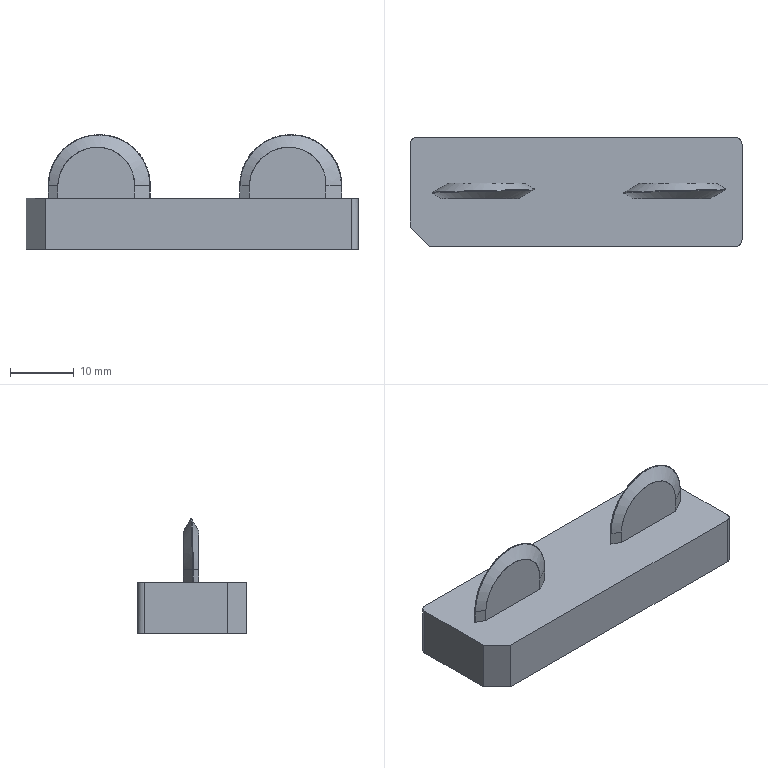NC program | PowerMill | posted with a generic post | part box 52 x 17 x 17.993 mm
Lines 9462 to 10240 of 175197:
N9559 M6
N9560 S8500 M03
N9561 G00 G90 X0.0 Y0.0
N9562 G43 Z9.7641 H3
N9563
N9564 G05 P10000 R8
N9565 X36.768 Y-7.8501
N9566 Z-8.99
N9567 G01 Z-10.19 F360.0
N9568 X31.4975 Y-7.6334 F600.0
N9569 Y0.5653
N9570 X28.8586 Y0.5675
N9571 X28.8583 Y0.2837
N9572 X28.8431 Y0.0
N9573 X28.8133 Y-0.2838
N9574 X28.7684 Y-0.5675
N9575 G02 X28.647 Y-1.0826 I-6.5218 J1.2655
N9576 G01 X28.5384 Y-1.4187
N9577 X28.4277 Y-1.7025
N9578 X28.2983 Y-1.9862
N9579 X28.1626 Y-2.2445
N9580 X28.0088 Y-2.5028
N9581 X27.779 Y-2.8375
N9582 X27.5532 Y-3.1213
N9583 X27.4447 Y-3.2451
N9584 X27.2187 Y-3.4806
N9585 X26.9945 Y-3.6887
N9586 X26.8771 Y-3.7891
N9587 X26.5942 Y-4.0081
N9588 X26.4095 Y-4.1344
N9589 X26.2217 Y-4.2562
N9590 X24.8539 Y-5.0498
N9591 X23.4821 Y-5.8366
N9592 X23.2337 Y-5.9587
N9593 X22.9163 Y-6.0931
N9594 X22.6334 Y-6.1934
N9595 X22.3504 Y-6.2763
N9596 X22.0675 Y-6.3429
N9597 X21.7846 Y-6.3935
N9598 X21.5017 Y-6.429
N9599 X21.2187 Y-6.4492
N9600 X20.6529 Y-6.455
N9601 X9.3363
N9602 X8.7704 Y-6.4517
N9603 X8.4875 Y-6.4344
N9604 X8.2046 Y-6.4021
N9605 G02 X7.6388 Y-6.2913 I0.9473 J6.3356
N9606 G01 X7.3558 Y-6.2118
N9607 X7.0602 Y-6.1105
N9608 X6.6972 Y-5.9588
N9609 X6.5071 Y-5.8667
N9610 X5.9412 Y-5.5486
N9611 X4.6897 Y-4.8238
N9612 X4.4667 Y-4.6794
N9613 X4.2437 Y-4.5184
N9614 X4.0631 Y-4.3751
N9615 X1.0968 Y-8.1713
N9616 G02 X0.7451 Y-9.1929 I-0.3518 J-0.4502
N9617 G01 X-0.7145 Y-9.193
N9618 G02 X-0.9257 Y-8.1556 I0.0 J0.5402
N9619 G01 X-0.3805 Y-7.924
N9620 G02 X0.5431 Y-7.9197 I0.467 J-1.0993
N9621 G01 X0.9635 Y-8.0936
N9622 G02 X1.0968 Y-8.1713 I-0.2185 J-0.528
N9623 G01 X4.0631 Y-4.3751
N9624 X3.923 Y-4.2563
N9625 X3.6779 Y-4.0257
N9626 X3.5166 Y-3.8572
N9627 X3.3685 Y-3.6887
N9628 G02 X2.9013 Y-3.0435 I4.0912 J3.4539
N9629 G01 X2.7769 Y-2.8375
N9630 X2.6286 Y-2.5538
N9631 X2.5463 Y-2.3764
N9632 X2.3904 Y-1.9863
N9633 G02 X2.2225 Y-1.4188 I6.0815 J2.1086
N9634 G01 X2.1632 Y-1.135
N9635 X2.1194 Y-0.8513
N9636 X2.0903 Y-0.5675
N9637 X2.076 Y-0.2838
N9638 X2.0764 Y0.0
N9639 X2.092 Y0.2838
N9640 X2.1225 Y0.5675
N9641 X2.1675 Y0.8512
N9642 X2.2278 Y1.135
N9643 X2.3048 Y1.4188
N9644 X2.3985 Y1.7025
N9645 X2.5098 Y1.9862
N9646 X2.6602 Y2.312
N9647 X2.7894 Y2.5537
N9648 G02 X3.1602 Y3.1213 I5.3365 J-3.0817
N9649 G01 X3.3863 Y3.405
N9650 X3.6779 Y3.7209
N9651 X3.9608 Y3.984
N9652 X4.2437 Y4.2144
N9653 G02 X4.8198 Y4.598 I3.727 J-4.9725
N9654 G01 X7.3959 Y6.0848
N9655 X7.6388 Y6.212
N9656 X7.9217 Y6.3406
N9657 X8.2046 Y6.4501
N9658 X8.3813 Y6.5085
N9659 X8.7704 Y6.6166
N9660 X9.0533 Y6.6754
N9661 X9.3362 Y6.7186
N9662 G02 X9.9021 Y6.7599 I0.7394 J-6.2346
N9663 G01 X21.7846 Y6.761
N9664 G02 X22.3504 Y6.7446 I0.0747 J-7.2155
N9665 G01 X22.6333 Y6.715
N9666 X22.9162 Y6.6701
N9667 G02 X23.5042 Y6.5262 I-1.2454 J-6.3649
N9668 G01 X23.776 Y6.4356
N9669 X24.0479 Y6.3281
N9670 X24.3308 Y6.1976
N9671 X24.6137 Y6.0466
N9672 X25.4638 Y5.5561
N9673 X26.3113 Y5.0612
N9674 X26.6561 Y4.8237
N9675 G02 X27.0908 Y4.4638 I-3.752 J-4.974
N9676 G01 X27.3045 Y4.2562
N9677 G02 X27.7869 Y3.6887 I-4.1486 J-4.0151
N9678 G01 X28.0087 Y3.3654
N9679 X28.1549 Y3.1213
N9680 X28.3041 Y2.8375
N9681 X28.4328 Y2.5538
N9682 X28.5746 Y2.178
N9683 X28.6354 Y1.9862
N9684 X28.7108 Y1.7025
N9685 X28.7708 Y1.4187
N9686 X28.8151 Y1.135
N9687 X28.8442 Y0.8512
N9688 X28.8586 Y0.5675
N9689 X31.4975 Y0.5653
N9690 G00 Z2.801
N9691 G01 X-36.768 Y7.8503 F10000.0
N9692 G00 Z-8.99
N9693 G01 Z-10.19 F360.0
N9694 X-31.4975 Y7.6335 F600.0
N9695 Y-0.5128
N9696 X-27.9215 Y-0.3548
N9697 X-27.9235 Y0.0
N9698 X-27.9079 Y0.2838
N9699 G02 X-27.8325 Y0.8513 I6.9347 J-0.6328
N9700 G01 X-27.7721 Y1.135
N9701 X-27.6952 Y1.4188
N9702 X-27.6015 Y1.7025
N9703 X-27.4905 Y1.9863
N9704 X-27.3336 Y2.324
N9705 G02 X-27.0541 Y2.8122 I5.6458 J-2.9085
N9706 G01 X-26.8398 Y3.1213
N9707 X-26.6139 Y3.405
N9708 X-26.3113 Y3.7317
N9709 X-26.0283 Y3.9934
N9710 X-25.7004 Y4.2563
N9711 X-25.44 Y4.438
N9712 X-25.1796 Y4.5982
N9713 X-22.5879 Y6.0946
N9714 X-22.4317 Y6.176
N9715 X-22.0675 Y6.3451
N9716 X-21.7846 Y6.4536
N9717 X-21.5636 Y6.5263
N9718 X-21.2188 Y6.6191
N9719 X-20.9358 Y6.6774
N9720 X-20.6529 Y6.7199
N9721 X-20.37 Y6.7475
N9722 X-20.1737 Y6.7568
N9723 X-19.5212 Y6.761
N9724 X-7.9217 Y6.7588
N9725 G02 X-7.3558 Y6.7135 I-0.2268 J-6.3843
N9726 G01 X-7.0729 Y6.6681
N9727 X-6.7866 Y6.6061
N9728 X-6.5071 Y6.5299
N9729 G02 X-5.9413 Y6.3234 I-1.9215 J-6.1454
N9730 G01 X-5.6583 Y6.1923
N9731 X-5.3754 Y6.0405
N9732 X-4.5252 Y5.55
N9733 X-3.6779 Y5.0543
N9734 X-3.3442 Y4.8237
N9735 X-3.0821 Y4.6152
N9736 X-2.9759 Y4.5221
N9737 X0.1585 Y8.1619
N9738 G02 X-0.0446 Y8.5772 I0.3827 J0.4444
N9739 G02 X0.5412 Y9.1928 I0.5858 J0.0291
N9740 G01 X1.205 Y9.1929
N9741 G02 X1.2599 Y8.0885 I0.0001 J-0.5536
N9742 G01 X0.5994 Y8.0227
N9743 G02 X0.1585 Y8.1619 I-0.0582 J0.5836
N9744 G01 X-2.9759 Y4.5221
N9745 X-2.9038 Y4.459
N9746 X-2.7215 Y4.2814
N9747 X-2.5463 Y4.0969
N9748 X-2.3711 Y3.8928
N9749 X-2.213 Y3.6887
N9750 X-1.9804 Y3.3482
N9751 X-1.8453 Y3.1213
N9752 X-1.6958 Y2.8375
N9753 X-1.5671 Y2.5537
N9754 X-1.4146 Y2.1456
N9755 X-1.3495 Y1.9287
N9756 X-1.2892 Y1.7025
N9757 X-1.2292 Y1.4187
N9758 X-1.1848 Y1.135
N9759 G02 X-1.1413 Y0.5675 I-6.6145 J-0.7918
N9760 G01 X-1.1416 Y0.2837
N9761 X-1.1569 Y0.0
N9762 G02 X-1.2314 Y-0.5675 I-6.5663 J0.5736
N9763 G01 X-1.2922 Y-0.8513
N9764 X-1.4146 Y-1.2813
N9765 X-1.4618 Y-1.4188
N9766 X-1.5722 Y-1.7025
N9767 X-1.7019 Y-1.9863
N9768 X-1.8325 Y-2.2359
N9769 X-2.0238 Y-2.5537
N9770 X-2.2209 Y-2.8375
N9771 X-2.4468 Y-3.1212
N9772 X-2.5463 Y-3.2349
N9773 X-2.7759 Y-3.4753
N9774 X-3.0054 Y-3.6888
N9775 X-3.1121 Y-3.7802
N9776 X-3.395 Y-4.0004
N9777 X-3.6779 Y-4.1939
N9778 X-3.878 Y-4.3143
N9779 X-5.191 Y-5.0752
N9780 X-6.5071 Y-5.8307
N9781 X-6.7665 Y-5.9588
N9782 X-7.0729 Y-6.0887
N9783 X-7.3558 Y-6.1896
N9784 X-7.6388 Y-6.2733
N9785 G02 X-8.2046 Y-6.3919 I-1.5816 J6.1369
N9786 G01 X-8.4875 Y-6.428
N9787 X-8.7704 Y-6.4489
N9788 X-9.3362 Y-6.455
N9789 X-20.6529
N9790 X-21.2188 Y-6.452
N9791 X-21.5017 Y-6.4354
N9792 G02 X-22.0675 Y-6.3568 I0.6091 J6.4567
N9793 G01 X-22.3504 Y-6.294
N9794 X-22.6334 Y-6.215
N9795 X-22.9163 Y-6.1192
N9796 X-23.3028 Y-5.9587
N9797 X-23.4821 Y-5.872
N9798 X-24.0479 Y-5.5547
N9799 X-25.3103 Y-4.8237
N9800 G02 X-26.1003 Y-4.2343 I2.9388 J4.7633
N9801 G01 X-26.3113 Y-4.0365
N9802 X-26.4747 Y-3.8656
N9803 X-26.6318 Y-3.6887
N9804 X-26.8771 Y-3.3756
N9805 X-27.0517 Y-3.1212
N9806 X-27.2229 Y-2.8375
N9807 X-27.3714 Y-2.5538
N9808 X-27.4429 Y-2.4005
N9809 X-27.5313 Y-2.1934
N9810 X-27.6095 Y-1.9863
N9811 X-27.7146 Y-1.6547
N9812 X-27.7775 Y-1.4187
N9813 X-27.8367 Y-1.135
N9814 X-27.8806 Y-0.8512
N9815 X-27.9057 Y-0.6034
N9816 X-27.9215 Y-0.3548
N9817 X-31.4975 Y-0.5128
N9818 G00 Z9.7641
N9819 G05 P0
N9820 (---------------)
N9821 ( END TOOLPATH : 精公基准台01-基准面偏置-D10 )
N9822 (---------------)
N9823 ( START TOOLPATH : 精公基准台01-基准台侧光-D10 )
N9824 (---------------)
N9825 G00 X0.0 Y0.0 Z9.7641
N9826 G05 P10000 R8
N9827 X30.2044 Y-17.2786
N9828 Z-16.89
N9829 G01 Z-18.09 F360.0
N9830 G03 X27.8526 Y-12.8662 I-1.1759 J2.2062 F600.0
N9831 G01 X27.7004 Y-12.9474
N9832 X27.6983 Y-12.9485
N9833 X27.6961 Y-12.9495
N9834 X27.38 Y-13.0947
N9835 X27.3779 Y-13.0957
N9836 X27.3758 Y-13.0965
N9837 X27.0597 Y-13.2205
N9838 X27.0576 Y-13.2213
N9839 X27.0554 Y-13.222
N9840 X26.7393 Y-13.3259
N9841 X26.7379 Y-13.3263
N9842 X26.7365 Y-13.3268
N9843 X26.6385 Y-13.355
N9844 X26.6375 Y-13.3553
N9845 X26.6364 Y-13.3555
N9846 X26.4183 Y-13.4122
N9847 X26.4164 Y-13.4127
N9848 X26.4146 Y-13.4131
N9849 X26.0984 Y-13.4794
N9850 X26.0965 Y-13.4798
N9851 X26.0945 Y-13.4802
N9852 X25.7783 Y-13.53
N9853 X25.7761 Y-13.5303
N9854 X25.7739 Y-13.5305
N9855 X25.4577 Y-13.5623
N9856 X25.4557 Y-13.5624
N9857 X25.4537 Y-13.5626
N9858 X25.1375 Y-13.5781
N9859 X25.1358 Y-13.5782
N9860 X25.134
N9861 X24.8179 Y-13.58
N9862 X24.8177
N9863 X24.8174
N9864 X-22.9206
N9865 X-22.9213
N9866 X-22.922
N9867 X-23.2381 Y-13.5744
N9868 X-23.2406 Y-13.5743
N9869 X-23.243 Y-13.5742
N9870 X-23.5592 Y-13.5491
N9871 X-23.5617 Y-13.5489
N9872 X-23.5642 Y-13.5485
N9873 X-23.8804 Y-13.5031
N9874 X-23.8829 Y-13.5027
N9875 X-23.8854 Y-13.5022
N9876 X-24.2016 Y-13.4358
N9877 X-24.204 Y-13.4353
N9878 X-24.2064 Y-13.4346
N9879 X-24.4942 Y-13.3552
N9880 X-24.4968 Y-13.3545
N9881 X-24.4993 Y-13.3537
N9882 X-24.8438 Y-13.2335
N9883 X-24.8464 Y-13.2326
N9884 X-24.8491 Y-13.2315
N9885 X-25.1652 Y-13.0954
N9886 X-25.167 Y-13.0946
N9887 X-25.1687 Y-13.0938
N9888 X-25.2914 Y-13.0338
N9889 X-25.2927 Y-13.0332
N9890 X-25.2939 Y-13.0326
N9891 X-25.4874 Y-12.9294
N9892 X-25.4894 Y-12.9282
N9893 X-25.4915 Y-12.927
N9894 X-25.8076 Y-12.7336
N9895 X-25.8102 Y-12.7319
N9896 X-25.8127 Y-12.7302
N9897 X-26.1288 Y-12.502
N9898 X-26.1306 Y-12.5007
N9899 X-26.1324 Y-12.4993
N9900 X-26.265 Y-12.3918
N9901 X-26.2663 Y-12.3908
N9902 X-26.2675 Y-12.3897
N9903 X-26.4511 Y-12.2278
N9904 X-26.4525 Y-12.2265
N9905 X-26.4538 Y-12.2253
N9906 X-26.6132 Y-12.071
N9907 X-26.6136 Y-12.0706
N9908 X-26.6141 Y-12.0701
N9909 X-29.6162 Y-9.0679
N9910 X-29.617 Y-9.067
N9911 X-29.6178 Y-9.0662
N9912 X-29.7681 Y-8.907
N9913 X-29.7694 Y-8.9056
N9914 X-29.7706 Y-8.9042
N9915 X-29.9365 Y-8.711
N9916 X-29.9375 Y-8.7097
N9917 X-29.9386 Y-8.7084
N9918 X-30.0356 Y-8.5855
N9919 X-30.0369 Y-8.5838
N9920 X-30.0382 Y-8.5821
N9921 X-30.2573 Y-8.2715
N9922 X-30.259 Y-8.269
N9923 X-30.2606 Y-8.2665
N9924 X-30.453 Y-7.9447
N9925 X-30.4545 Y-7.9422
N9926 X-30.4558 Y-7.9396
N9927 X-30.6149 Y-7.6234
N9928 X-30.6161 Y-7.6209
N9929 X-30.6172 Y-7.6184
N9930 X-30.7495 Y-7.3022
N9931 X-30.7505 Y-7.2997
N9932 X-30.7514 Y-7.2972
N9933 X-30.8593 Y-6.981
N9934 X-30.8599 Y-6.9792
N9935 X-30.8604 Y-6.9774
N9936 X-30.9011 Y-6.8363
N9937 X-30.9014 Y-6.8351
N9938 X-30.9018 Y-6.8338
N9939 X-30.9461 Y-6.6587
N9940 X-30.9466 Y-6.6567
N9941 X-30.947 Y-6.6548
N9942 X-31.0103 Y-6.3386
N9943 X-31.0107 Y-6.3361
N9944 X-31.0111 Y-6.3336
N9945 X-31.0536 Y-6.0174
N9946 X-31.0539 Y-6.0149
N9947 X-31.0541 Y-6.0123
N9948 X-31.0762 Y-5.6962
N9949 X-31.0763 Y-5.6939
N9950 X-31.0764 Y-5.6915
N9951 X-31.08 Y-5.3754
N9952 Y-5.3749
N9953 Y-5.3745
N9954 X-31.0792 Y7.5875
N9955 Y7.5891
N9956 Y7.5907
N9957 X-31.0664 Y7.9069
N9958 X-31.0662 Y7.909
N9959 X-31.0661 Y7.9112
N9960 X-31.0362 Y8.2273
N9961 X-31.036 Y8.2294
N9962 X-31.0357 Y8.2315
N9963 X-30.989 Y8.5476
N9964 X-30.9887 Y8.5498
N9965 X-30.9883 Y8.5519
N9966 X-30.924 Y8.868
N9967 X-30.9236 Y8.8701
N9968 X-30.9231 Y8.8722
N9969 X-30.8407 Y9.1884
N9970 X-30.8402 Y9.1905
N9971 X-30.8395 Y9.1926
N9972 X-30.7384 Y9.5087
N9973 X-30.7377 Y9.5108
N9974 X-30.7369 Y9.5129
N9975 X-30.6162 Y9.8291
N9976 X-30.6153 Y9.8312
N9977 X-30.6144 Y9.8333
N9978 X-30.4721 Y10.1495
N9979 X-30.4711 Y10.1516
N9980 X-30.4701 Y10.1537
N9981 X-30.3052 Y10.4698
N9982 X-30.304 Y10.4719
N9983 X-30.3028 Y10.4741
N9984 X-30.1126 Y10.7902
N9985 X-30.1113 Y10.7923
N9986 X-30.1099 Y10.7944
N9987 X-29.8918 Y11.1105
N9988 X-29.8903 Y11.1127
N9989 X-29.8887 Y11.1148
N9990 X-29.6383 Y11.4309
N9991 X-29.6365 Y11.4331
N9992 X-29.6347 Y11.4351
N9993 X-29.3464 Y11.7513
N9994 X-29.3444 Y11.7534
N9995 X-29.3423 Y11.7555
N9996 X-29.008 Y12.0717
N9997 X-29.0058 Y12.0737
N9998 X-29.0035 Y12.0756
N9999 X-28.6617 Y12.3536
N10000 X-28.6594 Y12.3554
N10001 X-28.6572 Y12.357
N10002 X-28.341 Y12.579
N10003 X-28.3394 Y12.5801
N10004 X-28.3377 Y12.5812
N10005 X-28.1281 Y12.7135
N10006 X-28.127 Y12.7142
N10007 X-28.1259 Y12.7148
N10008 X-28.0193 Y12.7773
N10009 X-28.0179 Y12.7781
N10010 X-28.0165 Y12.7789
N10011 X-27.7004 Y12.9474
N10012 X-27.6987 Y12.9482
N10013 X-27.6971 Y12.949
N10014 X-27.5176 Y13.0342
N10015 X-27.5166 Y13.0347
N10016 X-27.5155 Y13.0352
N10017 X-27.3788 Y13.0953
N10018 X-27.3773 Y13.0959
N10019 X-27.3758 Y13.0965
N10020 X-27.0597 Y13.2205
N10021 X-27.0576 Y13.2213
N10022 X-27.0554 Y13.222
N10023 X-26.7393 Y13.3259
N10024 X-26.7372 Y13.3266
N10025 X-26.7351 Y13.3272
N10026 X-26.4189 Y13.4121
N10027 X-26.4168 Y13.4126
N10028 X-26.4146 Y13.4131
N10029 X-26.0984 Y13.4794
N10030 X-26.0965 Y13.4798
N10031 X-26.0945 Y13.4802
N10032 X-25.7783 Y13.5299
N10033 X-25.7761 Y13.5303
N10034 X-25.7739 Y13.5305
N10035 X-25.4577 Y13.5623
N10036 X-25.4557 Y13.5624
N10037 X-25.4537 Y13.5626
N10038 X-25.1375 Y13.5781
N10039 X-25.1358 Y13.5782
N10040 X-25.134
N10041 X-24.8179 Y13.58
N10042 X-24.8177
N10043 X-24.8174
N10044 X0.0
N10045 X24.8174
N10046 X24.8177
N10047 X24.8179
N10048 X25.134 Y13.5782
N10049 X25.1357
N10050 X25.1374 Y13.5781
N10051 X25.4535 Y13.563
N10052 X25.4557 Y13.5629
N10053 X25.4578 Y13.5627
N10054 X25.774 Y13.5305
N10055 X25.7761 Y13.5303
N10056 X25.7782 Y13.53
N10057 X26.0943 Y13.4807
N10058 X26.0965 Y13.4803
N10059 X26.0985 Y13.4799
N10060 X26.4147 Y13.4131
N10061 X26.4168 Y13.4126
N10062 X26.4189 Y13.4121
N10063 X26.7351 Y13.3271
N10064 X26.7372 Y13.3265
N10065 X26.7394 Y13.3259
N10066 X27.0555 Y13.2216
N10067 X27.0576 Y13.2209
N10068 X27.0596 Y13.2201
N10069 X27.3757 Y13.0966
N10070 X27.3773 Y13.0959
N10071 X27.3788 Y13.0953
N10072 X27.5154 Y13.0352
N10073 X27.5166 Y13.0347
N10074 X27.5177 Y13.0342
N10075 X27.6972 Y12.9485
N10076 X27.6988 Y12.9478
N10077 X27.7003 Y12.947
N10078 X28.0164 Y12.7789
N10079 X28.0179 Y12.7781
N10080 X28.0193 Y12.7773
N10081 X28.1259 Y12.7148
N10082 X28.1269 Y12.7142
N10083 X28.128 Y12.7136
N10084 X28.3376 Y12.582
N10085 X28.3392 Y12.5809
N10086 X28.3408 Y12.5799
N10087 X28.6058 Y12.3953
N10088 X28.6079 Y12.3938
N10089 X28.61 Y12.3922
N10090 X28.9773 Y12.0985
N10091 X28.9796 Y12.0966
N10092 X28.9818 Y12.0946
N10093 X29.298 Y11.8004
N10094 X29.3002 Y11.7983
N10095 X29.3023 Y11.7961
N10096 X29.6184 Y11.4537
N10097 X29.6203 Y11.4515
N10098 X29.6222 Y11.4492
N10099 X29.8885 Y11.1149
N10100 X29.8902 Y11.1128
N10101 X29.8918 Y11.1105
N10102 X30.1097 Y10.7944
N10103 X30.1109 Y10.7926
N10104 X30.1121 Y10.7907
N10105 X30.2601 Y10.5491
N10106 X30.2614 Y10.547
N10107 X30.2626 Y10.5449
N10108 X30.47 Y10.1542
N10109 X30.4711 Y10.1521
N10110 X30.4721 Y10.15
N10111 X30.5808 Y9.9125
N10112 X30.5817 Y9.9104
N10113 X30.5826 Y9.9083
N10114 X30.7368 Y9.5135
N10115 X30.7377 Y9.5111
N10116 X30.7385 Y9.5087
N10117 X30.8396 Y9.1926
N10118 X30.8403 Y9.1905
N10119 X30.8408 Y9.1884
N10120 X30.9231 Y8.8722
N10121 X30.9236 Y8.87
N10122 X30.9241 Y8.8678
N10123 X30.9876 Y8.5517
N10124 X30.9879 Y8.5497
N10125 X30.9883 Y8.5478
N10126 X31.0357 Y8.2317
N10127 X31.036 Y8.2294
N10128 X31.0363 Y8.2271
N10129 X31.0653 Y7.911
N10130 X31.0655 Y7.909
N10131 X31.0656 Y7.9071
N10132 X31.0792 Y7.5909
N10133 Y7.5892
N10134 Y7.5875
N10135 Y-7.5875
N10136 Y-7.5891
N10137 Y-7.5907
N10138 X31.0664 Y-7.9069
N10139 X31.0662 Y-7.909
N10140 X31.0661 Y-7.9112
N10141 X31.0362 Y-8.2273
N10142 X31.036 Y-8.2294
N10143 X31.0357 Y-8.2315
N10144 X30.989 Y-8.5476
N10145 X30.9887 Y-8.5498
N10146 X30.9883 Y-8.5519
N10147 X30.924 Y-8.868
N10148 X30.9236 Y-8.8701
N10149 X30.9231 Y-8.8722
N10150 X30.8407 Y-9.1884
N10151 X30.8402 Y-9.1905
N10152 X30.8395 Y-9.1926
N10153 X30.7384 Y-9.5087
N10154 X30.7377 Y-9.5108
N10155 X30.7369 Y-9.5129
N10156 X30.6162 Y-9.8291
N10157 X30.6153 Y-9.8312
N10158 X30.6144 Y-9.8333
N10159 X30.4721 Y-10.1495
N10160 X30.4711 Y-10.1516
N10161 X30.4701 Y-10.1537
N10162 X30.3052 Y-10.4698
N10163 X30.304 Y-10.4719
N10164 X30.3028 Y-10.4741
N10165 X30.1126 Y-10.7902
N10166 X30.1113 Y-10.7923
N10167 X30.1099 Y-10.7944
N10168 X29.8918 Y-11.1105
N10169 X29.8903 Y-11.1127
N10170 X29.8887 Y-11.1148
N10171 X29.6383 Y-11.4309
N10172 X29.6365 Y-11.4331
N10173 X29.6347 Y-11.4351
N10174 X29.3464 Y-11.7513
N10175 X29.3444 Y-11.7534
N10176 X29.3423 Y-11.7555
N10177 X29.008 Y-12.0717
N10178 X29.0058 Y-12.0737
N10179 X29.0035 Y-12.0756
N10180 X28.6617 Y-12.3536
N10181 X28.6594 Y-12.3554
N10182 X28.6572 Y-12.357
N10183 X28.341 Y-12.579
N10184 X28.3394 Y-12.5801
N10185 X28.3377 Y-12.5812
N10186 X28.1281 Y-12.7135
N10187 X28.127 Y-12.7142
N10188 X28.1259 Y-12.7148
N10189 X28.0193 Y-12.7773
N10190 X28.0179 Y-12.7781
N10191 X28.0165 Y-12.7789
N10192 X27.8526 Y-12.8662
N10193 G03 X30.2043 Y-17.2787 I1.1759 J-2.2062
N10194 G01 X30.1567 Y-17.2134
N10195 G03 X27.805 Y-12.801 I-1.1759 J2.2062
N10196 G01 X27.6627 Y-12.8768
N10197 X27.3466 Y-13.022
N10198 X27.0305 Y-13.146
N10199 X26.7143 Y-13.2499
N10200 X26.6163 Y-13.2781
N10201 X26.3982 Y-13.3348
N10202 X26.082 Y-13.4012
N10203 X25.7659 Y-13.4509
N10204 X25.4497 Y-13.4827
N10205 X25.1336 Y-13.4982
N10206 X24.8174 Y-13.5
N10207 X-22.9206
N10208 X-23.2367 Y-13.4944
N10209 X-23.5529 Y-13.4694
N10210 X-23.869 Y-13.4239
N10211 X-24.1851 Y-13.3575
N10212 X-24.473 Y-13.2781
N10213 X-24.8174 Y-13.158
N10214 X-25.1336 Y-13.0219
N10215 X-25.2563 Y-12.962
N10216 X-25.4497 Y-12.8588
N10217 X-25.7659 Y-12.6653
N10218 X-26.082 Y-12.4372
N10219 X-26.2146 Y-12.3297
N10220 X-26.3982 Y-12.1678
N10221 X-26.5575 Y-12.0135
N10222 X-29.5596 Y-9.0113
N10223 X-29.7099 Y-8.8521
N10224 X-29.8758 Y-8.6589
N10225 X-29.9728 Y-8.5359
N10226 X-30.1919 Y-8.2254
N10227 X-30.3844 Y-7.9036
N10228 X-30.5434 Y-7.5875
N10229 X-30.6757 Y-7.2714
N10230 X-30.7836 Y-6.9552
N10231 X-30.8242 Y-6.8142
N10232 X-30.8685 Y-6.6391
N10233 X-30.9318 Y-6.3229
N10234 X-30.9743 Y-6.0068
N10235 X-30.9964 Y-5.6906
N10236 X-31.0 Y-5.3745
N10237 Y7.2714
N10238 X-30.9992 Y7.5875
N10239 X-30.9864 Y7.9036
N10240 X-30.9566 Y8.2198
N10241 X-30.9099 Y8.5359
N10242 X-30.8456 Y8.8521
N10243 X-30.7633 Y9.1682
N10244 X-30.6622 Y9.4844
N10245 X-30.5415 Y9.8005
N10246 X-30.3992 Y10.1167
N10247 X-30.2343 Y10.4328
N10248 X-30.044 Y10.749
N10249 X-29.8259 Y11.0651
N10250 X-29.5756 Y11.3812
N10251 X-29.2873 Y11.6974
N10252 X-28.9531 Y12.0135
N10253 X-28.6112 Y12.2915
N10254 X-28.295 Y12.5135
N10255 X-28.0854 Y12.6458
N10256 X-27.9789 Y12.7083
N10257 X-27.6627 Y12.8768
N10258 X-27.4833 Y12.962
N10259 X-27.3466 Y13.022
N10260 X-27.0305 Y13.146
N10261 X-26.7143 Y13.2499
N10262 X-26.3982 Y13.3348
N10263 X-26.082 Y13.4012
N10264 X-25.7659 Y13.4509
N10265 X-25.4497 Y13.4826
N10266 X-25.1336 Y13.4982
N10267 X-24.8174 Y13.5
N10268 X0.0
N10269 X24.8174
N10270 X25.1336 Y13.4982
N10271 X25.4497 Y13.4831
N10272 X25.7659 Y13.4509
N10273 X26.082 Y13.4016
N10274 X26.3982 Y13.3348
N10275 X26.7143 Y13.2499
N10276 X27.0305 Y13.1456
N10277 X27.3466 Y13.022
N10278 X27.4832 Y12.962
N10279 X27.6627 Y12.8763
N10280 X27.9789 Y12.7083
N10281 X28.0854 Y12.6458
N10282 X28.295 Y12.5142
N10283 X28.56 Y12.3297
N10284 X28.9273 Y12.0361
N10285 X29.2435 Y11.7418
N10286 X29.5596 Y11.3994
N10287 X29.8259 Y11.0651
N10288 X30.0439 Y10.749
N10289 X30.1919 Y10.5073
N10290 X30.3993 Y10.1167
N10291 X30.5081 Y9.8792
N10292 X30.6623 Y9.4844
N10293 X30.7634 Y9.1682
N10294 X30.8457 Y8.8521
N10295 X30.9091 Y8.5359
N10296 X30.9566 Y8.2198
N10297 X30.9857 Y7.9036
N10298 X30.9992 Y7.5875
N10299 X31.0 Y7.2714
N10300 Y-7.2714
N10301 X30.9992 Y-7.5875
N10302 X30.9864 Y-7.9036
N10303 X30.9566 Y-8.2198
N10304 X30.9099 Y-8.5359
N10305 X30.8456 Y-8.8521
N10306 X30.7633 Y-9.1682
N10307 X30.6622 Y-9.4844
N10308 X30.5415 Y-9.8005
N10309 X30.3992 Y-10.1167
N10310 X30.2343 Y-10.4328
N10311 X30.044 Y-10.749
N10312 X29.8259 Y-11.0651
N10313 X29.5756 Y-11.3812
N10314 X29.2873 Y-11.6974
N10315 X28.9531 Y-12.0135
N10316 X28.6112 Y-12.2915
N10317 X28.295 Y-12.5135
N10318 X28.0854 Y-12.6458
N10319 X27.9789 Y-12.7083
N10320 X27.805 Y-12.801
N10321 G03 X30.1567 Y-17.2134 I1.1758 J-2.2062
N10322 G00 Z9.7641
N10323 G05 P0
N10324 (---------------)
N10325 ( END TOOLPATH : 精公基准台01-基准台侧光-D10 )
N10326 (---------------)
N10327
N10328 M05
N10329 G53 Z0.0
N10330 (---------------)
N10331 ( START TOOLPATH : 精公精光01-浅滩和陡峭-R1 )
N10332 (---------------)
N10333 ( TOOL NO.    :4 )
N10334 ( TOOL TYPE   : BALLNOSED)
N10335 ( TOOL ID     : R1_1_1)
N10336 ( TOOL DIA    : 2.0 LENGTH 64.4)
N10337 T4